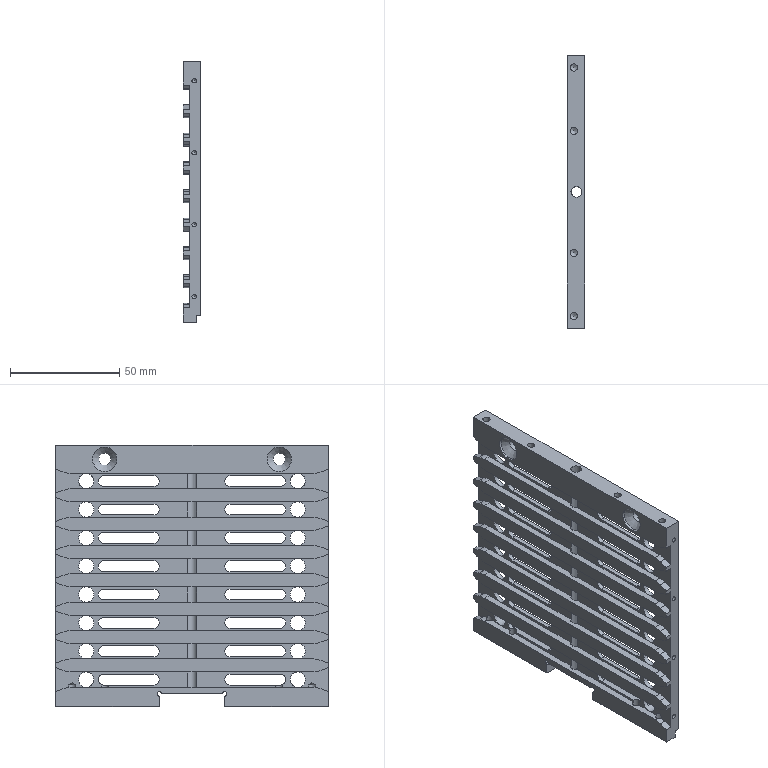Part | 1 solid | 283 faces | box 8 x 125 x 120 mm | volume 58521 mm3 | plane 146 | cylinder 119 | cone 18 | commonest cylinder face diameters 20 x44 5 x33 7 x16 2.05 x8 3.3 x8 2 x6